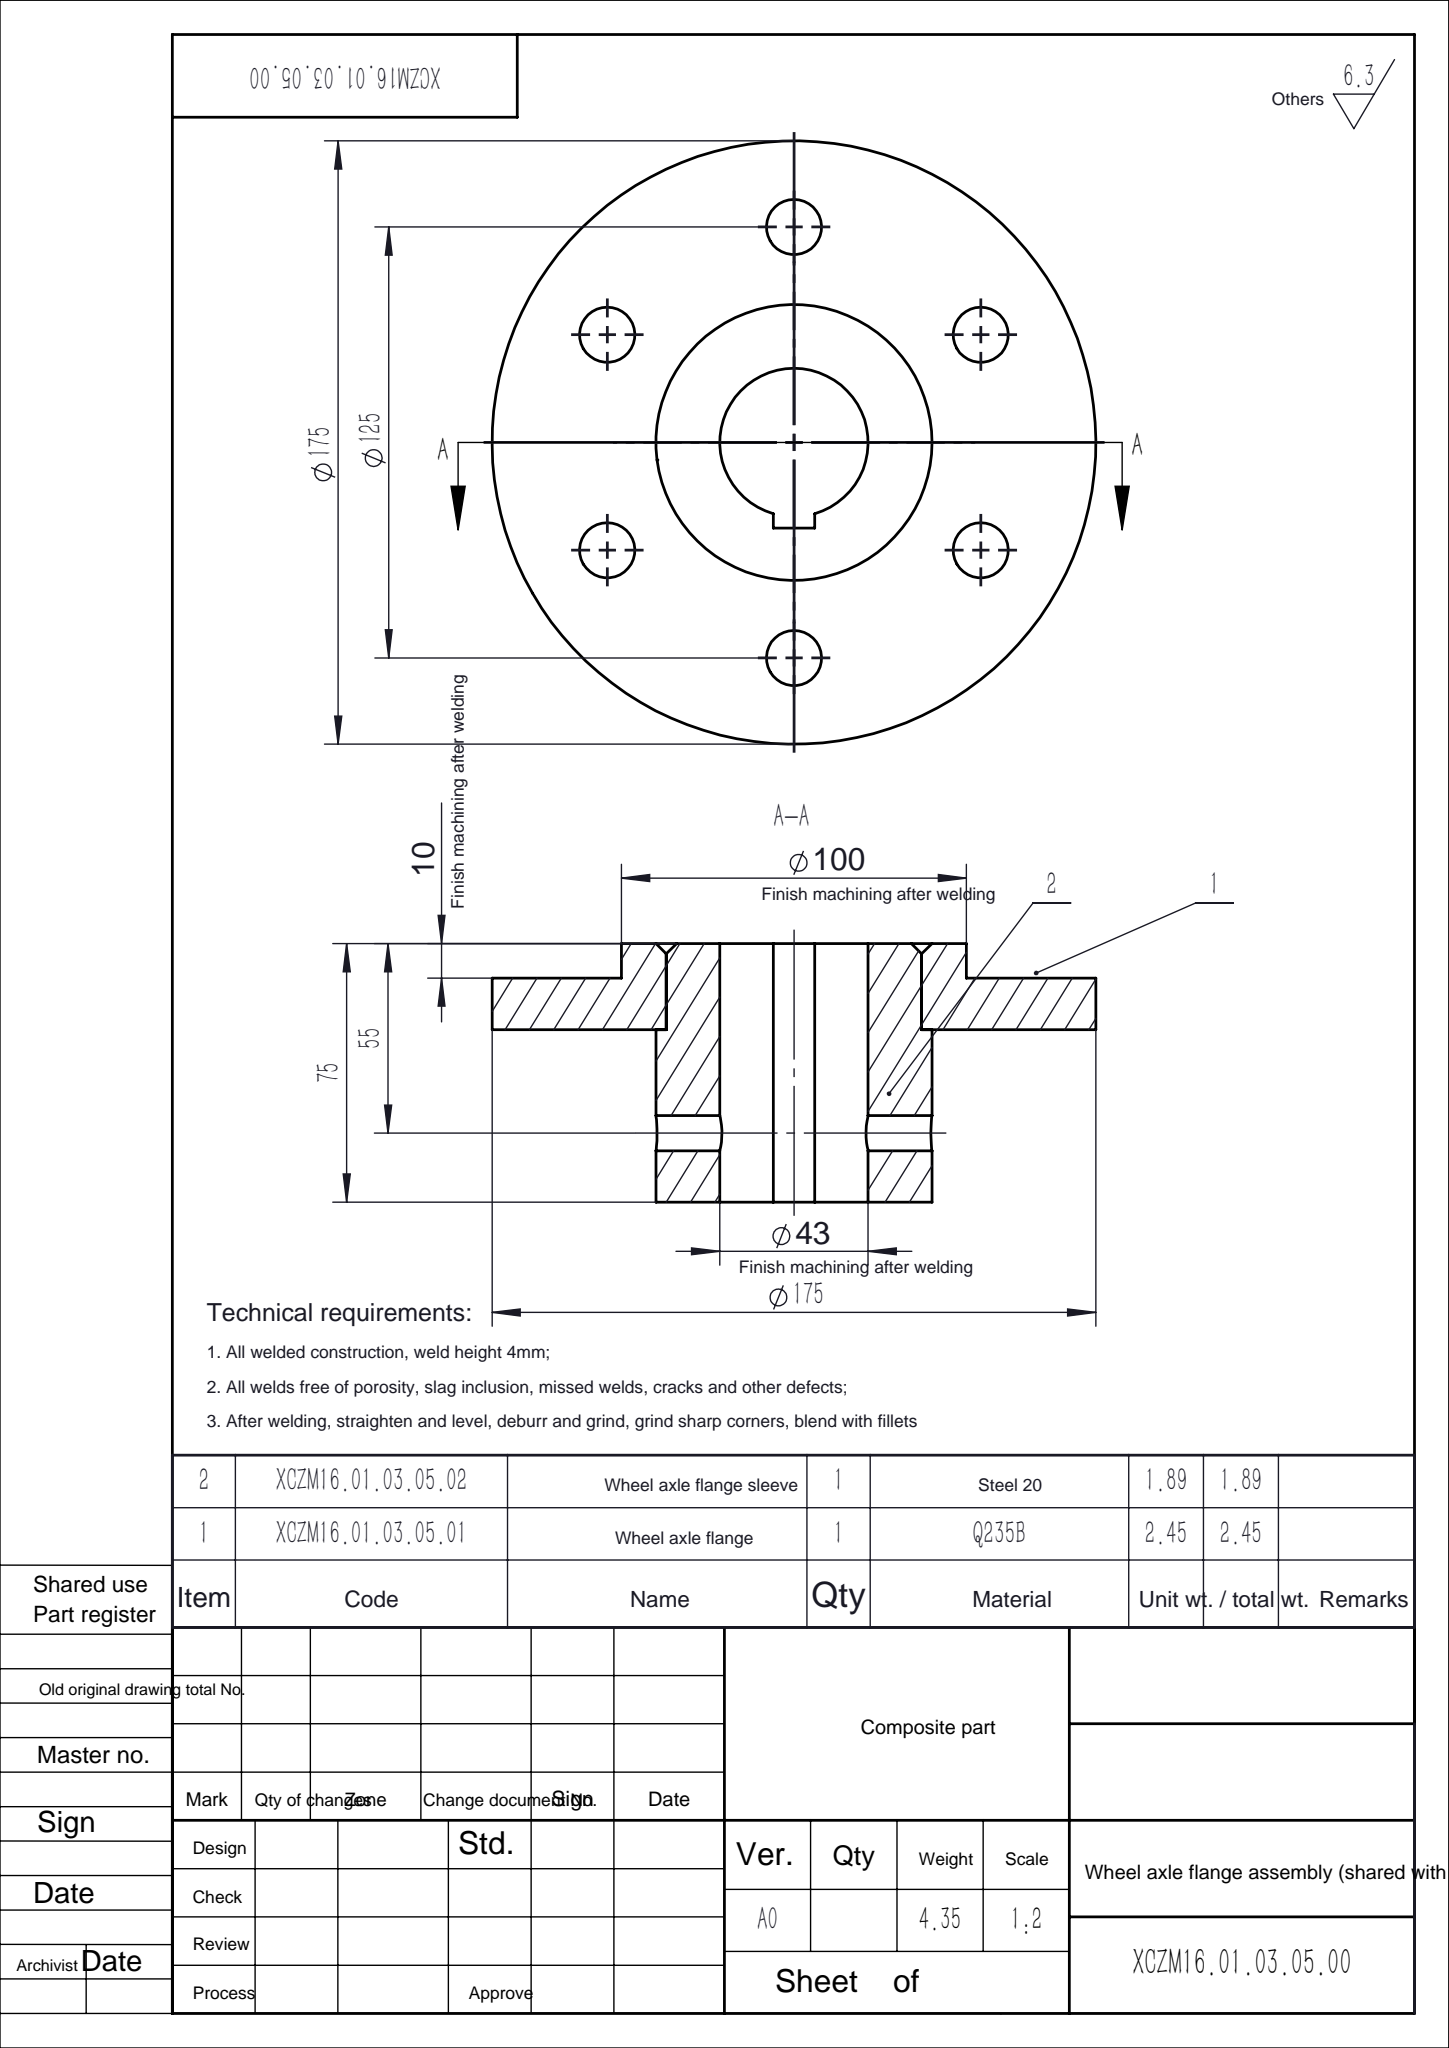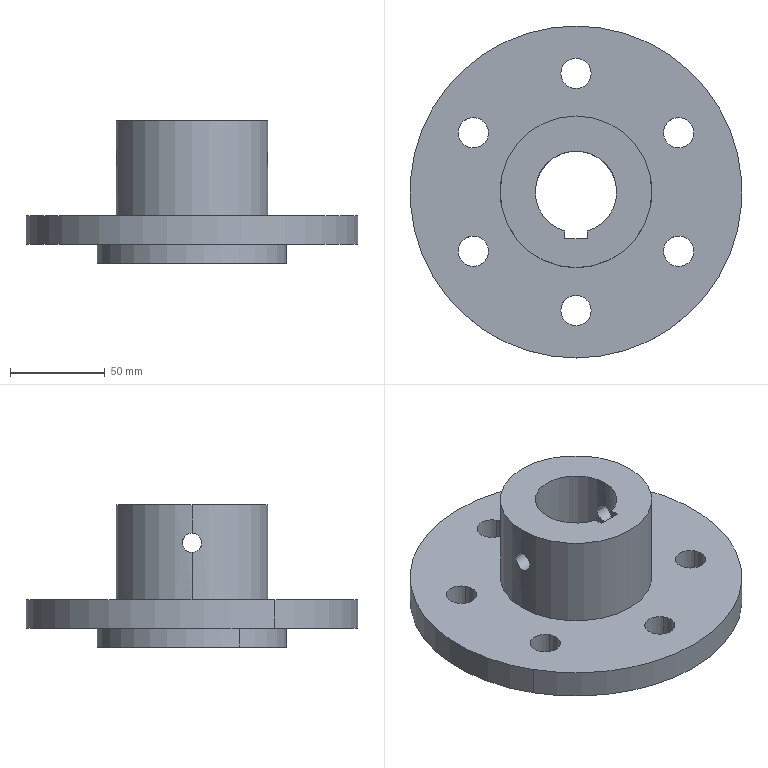Part | SolidWorks | 2 solids | 42 faces | box 175 x 175 x 75 mm | volume 555297 mm3 | cylinder 29 | plane 9 | cone 4 | commonest cylinder face diameters 16 x12 10.2 x4 74 x4 43 x3 80 x2 100 x2